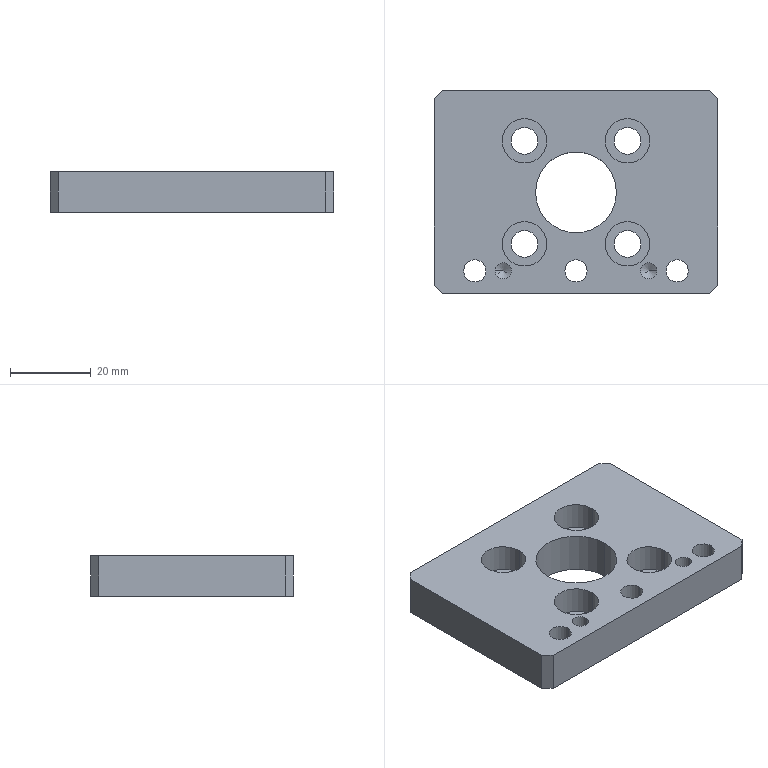Part | SolidWorks | features HoleWzd 3, Chamfer 1, Extrusion 1, ICE 1 | 1 solid | 46 faces | box 70 x 50 x 10 mm | volume 27882 mm3 | cylinder 28 | plane 14 | cone 4 | commonest cylinder face diameters 6.6 x8 11 x8 5.5 x6 4 x4 20 x2
STEP:
#1=CARTESIAN_POINT('',(-20.,-19.5,4.));
#2=VERTEX_POINT('',#1);
#3=CARTESIAN_POINT('',(-16.,-19.5,4.));
#4=VERTEX_POINT('',#3);
#5=CARTESIAN_POINT('',(-18.,-19.5,4.));
#6=DIRECTION('',(0.,0.,1.));
#7=DIRECTION('',(1.,0.,0.));
#8=AXIS2_PLACEMENT_3D('',#5,#6,#7);
#9=CIRCLE('',#8,2.);
#10=EDGE_CURVE('',#2,#4,#9,.T.);
#11=ORIENTED_EDGE('',*,*,#10,.F.);
#12=CARTESIAN_POINT('',(-20.,-19.5,10.));
#13=VERTEX_POINT('',#12);
#14=CARTESIAN_POINT('',(-20.,-19.5,10.));
#15=DIRECTION('',(0.,0.,1.));
#16=VECTOR('',#15,1000.);
#17=LINE('',#14,#16);
#18=EDGE_CURVE('',#2,#13,#17,.T.);
#19=ORIENTED_EDGE('',*,*,#18,.T.);
#20=CARTESIAN_POINT('',(-16.,-19.5,10.));
#21=VERTEX_POINT('',#20);
#22=CARTESIAN_POINT('',(-18.,-19.5,10.));
#23=DIRECTION('',(0.,0.,1.));
#24=DIRECTION('',(1.,0.,0.));
#25=AXIS2_PLACEMENT_3D('',#22,#23,#24);
#26=CIRCLE('',#25,2.);
#27=EDGE_CURVE('',#13,#21,#26,.T.);
#28=ORIENTED_EDGE('',*,*,#27,.T.);
#29=CARTESIAN_POINT('',(-16.,-19.5,10.));
#30=DIRECTION('',(0.,0.,1.));
#31=VECTOR('',#30,1000.);
#32=LINE('',#29,#31);
#33=EDGE_CURVE('',#4,#21,#32,.T.);
#34=ORIENTED_EDGE('',*,*,#33,.F.);
#35=EDGE_LOOP('',(#11,#19,#28,#34));
#36=FACE_OUTER_BOUND('',#35,.T.);
#37=CARTESIAN_POINT('',(-18.,-19.5,10.));
#38=DIRECTION('',(0.,0.,1.));
#39=DIRECTION('',(1.,0.,0.));
#40=AXIS2_PLACEMENT_3D('',#37,#38,#39);
#41=CYLINDRICAL_SURFACE('',#40,2.);
#42=ADVANCED_FACE('',(#36),#41,.F.);
#43=CARTESIAN_POINT('',(-18.,-19.5,2.798));
#44=VERTEX_POINT('',#43);
#45=CARTESIAN_POINT('',(-16.,-19.5,4.));
#46=DIRECTION('',(0.8572,0.,0.515));
#47=VECTOR('',#46,1000.);
#48=LINE('',#45,#47);
#49=EDGE_CURVE('',#44,#4,#48,.T.);
#50=ORIENTED_EDGE('',*,*,#49,.F.);
#51=CARTESIAN_POINT('',(-20.,-19.5,4.));
#52=DIRECTION('',(-0.8572,0.,0.515));
#53=VECTOR('',#52,1000.);
#54=LINE('',#51,#53);
#55=EDGE_CURVE('',#44,#2,#54,.T.);
#56=ORIENTED_EDGE('',*,*,#55,.T.);
#57=ORIENTED_EDGE('',*,*,#10,.T.);
#58=EDGE_LOOP('',(#50,#56,#57));
#59=FACE_OUTER_BOUND('',#58,.T.);
#60=CARTESIAN_POINT('',(-18.,-19.5,4.));
#61=DIRECTION('',(0.,0.,1.));
#62=DIRECTION('',(1.,0.,0.));
#63=AXIS2_PLACEMENT_3D('',#60,#61,#62);
#64=CONICAL_SURFACE('',#63,2.,1.03);
#65=ADVANCED_FACE('',(#59),#64,.F.);
#66=CARTESIAN_POINT('',(16.,-19.5,4.));
#67=VERTEX_POINT('',#66);
#68=CARTESIAN_POINT('',(20.,-19.5,4.));
#69=VERTEX_POINT('',#68);
#70=CARTESIAN_POINT('',(18.,-19.5,4.));
#71=DIRECTION('',(0.,0.,1.));
#72=DIRECTION('',(1.,0.,0.));
#73=AXIS2_PLACEMENT_3D('',#70,#71,#72);
#74=CIRCLE('',#73,2.);
#75=EDGE_CURVE('',#67,#69,#74,.T.);
#76=ORIENTED_EDGE('',*,*,#75,.F.);
#77=CARTESIAN_POINT('',(16.,-19.5,10.));
#78=VERTEX_POINT('',#77);
#79=CARTESIAN_POINT('',(16.,-19.5,10.));
#80=DIRECTION('',(0.,0.,1.));
#81=VECTOR('',#80,1000.);
#82=LINE('',#79,#81);
#83=EDGE_CURVE('',#67,#78,#82,.T.);
#84=ORIENTED_EDGE('',*,*,#83,.T.);
#85=CARTESIAN_POINT('',(20.,-19.5,10.));
#86=VERTEX_POINT('',#85);
#87=CARTESIAN_POINT('',(18.,-19.5,10.));
#88=DIRECTION('',(0.,0.,1.));
#89=DIRECTION('',(1.,0.,0.));
#90=AXIS2_PLACEMENT_3D('',#87,#88,#89);
#91=CIRCLE('',#90,2.);
#92=EDGE_CURVE('',#78,#86,#91,.T.);
#93=ORIENTED_EDGE('',*,*,#92,.T.);
#94=CARTESIAN_POINT('',(20.,-19.5,10.));
#95=DIRECTION('',(0.,0.,1.));
#96=VECTOR('',#95,1000.);
#97=LINE('',#94,#96);
#98=EDGE_CURVE('',#69,#86,#97,.T.);
#99=ORIENTED_EDGE('',*,*,#98,.F.);
#100=EDGE_LOOP('',(#76,#84,#93,#99));
#101=FACE_OUTER_BOUND('',#100,.T.);
#102=CARTESIAN_POINT('',(18.,-19.5,10.));
#103=DIRECTION('',(0.,0.,1.));
#104=DIRECTION('',(1.,0.,0.));
#105=AXIS2_PLACEMENT_3D('',#102,#103,#104);
#106=CYLINDRICAL_SURFACE('',#105,2.);
#107=ADVANCED_FACE('',(#101),#106,.F.);
#108=CARTESIAN_POINT('',(18.,-19.5,2.798));
#109=VERTEX_POINT('',#108);
#110=CARTESIAN_POINT('',(20.,-19.5,4.));
#111=DIRECTION('',(0.8572,0.,0.515));
#112=VECTOR('',#111,1000.);
#113=LINE('',#110,#112);
#114=EDGE_CURVE('',#109,#69,#113,.T.);
#115=ORIENTED_EDGE('',*,*,#114,.F.);
#116=CARTESIAN_POINT('',(16.,-19.5,4.));
#117=DIRECTION('',(-0.8572,0.,0.515));
#118=VECTOR('',#117,1000.);
#119=LINE('',#116,#118);
#120=EDGE_CURVE('',#109,#67,#119,.T.);
#121=ORIENTED_EDGE('',*,*,#120,.T.);
#122=ORIENTED_EDGE('',*,*,#75,.T.);
#123=EDGE_LOOP('',(#115,#121,#122));
#124=FACE_OUTER_BOUND('',#123,.T.);
#125=CARTESIAN_POINT('',(18.,-19.5,4.));
#126=DIRECTION('',(0.,0.,1.));
#127=DIRECTION('',(1.,0.,0.));
#128=AXIS2_PLACEMENT_3D('',#125,#126,#127);
#129=CONICAL_SURFACE('',#128,2.,1.03);
#130=ADVANCED_FACE('',(#124),#129,.F.);
#131=CARTESIAN_POINT('',(-27.75,-19.5,0.));
#132=VERTEX_POINT('',#131);
#133=CARTESIAN_POINT('',(-22.25,-19.5,0.));
#134=VERTEX_POINT('',#133);
#135=CARTESIAN_POINT('',(-25.,-19.5,0.));
#136=DIRECTION('',(0.,0.,1.));
#137=DIRECTION('',(1.,0.,0.));
#138=AXIS2_PLACEMENT_3D('',#135,#136,#137);
#139=CIRCLE('',#138,2.75);
#140=EDGE_CURVE('',#132,#134,#139,.T.);
#141=ORIENTED_EDGE('',*,*,#140,.F.);
#142=CARTESIAN_POINT('',(-27.75,-19.5,10.));
#143=VERTEX_POINT('',#142);
#144=CARTESIAN_POINT('',(-27.75,-19.5,10.));
#145=DIRECTION('',(0.,0.,1.));
#146=VECTOR('',#145,1000.);
#147=LINE('',#144,#146);
#148=EDGE_CURVE('',#132,#143,#147,.T.);
#149=ORIENTED_EDGE('',*,*,#148,.T.);
#150=CARTESIAN_POINT('',(-22.25,-19.5,10.));
#151=VERTEX_POINT('',#150);
#152=CARTESIAN_POINT('',(-25.,-19.5,10.));
#153=DIRECTION('',(0.,0.,1.));
#154=DIRECTION('',(1.,0.,0.));
#155=AXIS2_PLACEMENT_3D('',#152,#153,#154);
#156=CIRCLE('',#155,2.75);
#157=EDGE_CURVE('',#143,#151,#156,.T.);
#158=ORIENTED_EDGE('',*,*,#157,.T.);
#159=CARTESIAN_POINT('',(-22.25,-19.5,10.));
#160=DIRECTION('',(0.,0.,1.));
#161=VECTOR('',#160,1000.);
#162=LINE('',#159,#161);
#163=EDGE_CURVE('',#134,#151,#162,.T.);
#164=ORIENTED_EDGE('',*,*,#163,.F.);
#165=EDGE_LOOP('',(#141,#149,#158,#164));
#166=FACE_OUTER_BOUND('',#165,.T.);
#167=CARTESIAN_POINT('',(-25.,-19.5,10.));
#168=DIRECTION('',(0.,0.,1.));
#169=DIRECTION('',(1.,0.,0.));
#170=AXIS2_PLACEMENT_3D('',#167,#168,#169);
#171=CYLINDRICAL_SURFACE('',#170,2.75);
#172=ADVANCED_FACE('',(#166),#171,.F.);
#173=CARTESIAN_POINT('',(-2.75,-19.5,0.));
#174=VERTEX_POINT('',#173);
#175=CARTESIAN_POINT('',(2.75,-19.5,0.));
#176=VERTEX_POINT('',#175);
#177=CARTESIAN_POINT('',(0.,-19.5,0.));
#178=DIRECTION('',(0.,0.,1.));
#179=DIRECTION('',(1.,0.,0.));
#180=AXIS2_PLACEMENT_3D('',#177,#178,#179);
#181=CIRCLE('',#180,2.75);
#182=EDGE_CURVE('',#174,#176,#181,.T.);
#183=ORIENTED_EDGE('',*,*,#182,.F.);
#184=CARTESIAN_POINT('',(-2.75,-19.5,10.));
#185=VERTEX_POINT('',#184);
#186=CARTESIAN_POINT('',(-2.75,-19.5,10.));
#187=DIRECTION('',(0.,0.,1.));
#188=VECTOR('',#187,1000.);
#189=LINE('',#186,#188);
#190=EDGE_CURVE('',#174,#185,#189,.T.);
#191=ORIENTED_EDGE('',*,*,#190,.T.);
#192=CARTESIAN_POINT('',(2.75,-19.5,10.));
#193=VERTEX_POINT('',#192);
#194=CARTESIAN_POINT('',(0.,-19.5,10.));
#195=DIRECTION('',(0.,0.,1.));
#196=DIRECTION('',(1.,0.,0.));
#197=AXIS2_PLACEMENT_3D('',#194,#195,#196);
#198=CIRCLE('',#197,2.75);
#199=EDGE_CURVE('',#185,#193,#198,.T.);
#200=ORIENTED_EDGE('',*,*,#199,.T.);
#201=CARTESIAN_POINT('',(2.75,-19.5,10.));
#202=DIRECTION('',(0.,0.,1.));
#203=VECTOR('',#202,1000.);
#204=LINE('',#201,#203);
#205=EDGE_CURVE('',#176,#193,#204,.T.);
#206=ORIENTED_EDGE('',*,*,#205,.F.);
#207=EDGE_LOOP('',(#183,#191,#200,#206));
#208=FACE_OUTER_BOUND('',#207,.T.);
#209=CARTESIAN_POINT('',(0.,-19.5,10.));
#210=DIRECTION('',(0.,0.,1.));
#211=DIRECTION('',(1.,0.,0.));
#212=AXIS2_PLACEMENT_3D('',#209,#210,#211);
#213=CYLINDRICAL_SURFACE('',#212,2.75);
#214=ADVANCED_FACE('',(#208),#213,.F.);
#215=CARTESIAN_POINT('',(22.25,-19.5,0.));
#216=VERTEX_POINT('',#215);
#217=CARTESIAN_POINT('',(27.75,-19.5,0.));
#218=VERTEX_POINT('',#217);
#219=CARTESIAN_POINT('',(25.,-19.5,0.));
#220=DIRECTION('',(0.,0.,1.));
#221=DIRECTION('',(1.,0.,0.));
#222=AXIS2_PLACEMENT_3D('',#219,#220,#221);
#223=CIRCLE('',#222,2.75);
#224=EDGE_CURVE('',#216,#218,#223,.T.);
#225=ORIENTED_EDGE('',*,*,#224,.F.);
#226=CARTESIAN_POINT('',(22.25,-19.5,10.));
#227=VERTEX_POINT('',#226);
#228=CARTESIAN_POINT('',(22.25,-19.5,10.));
#229=DIRECTION('',(0.,0.,1.));
#230=VECTOR('',#229,1000.);
#231=LINE('',#228,#230);
#232=EDGE_CURVE('',#216,#227,#231,.T.);
#233=ORIENTED_EDGE('',*,*,#232,.T.);
#234=CARTESIAN_POINT('',(27.75,-19.5,10.));
#235=VERTEX_POINT('',#234);
#236=CARTESIAN_POINT('',(25.,-19.5,10.));
#237=DIRECTION('',(0.,0.,1.));
#238=DIRECTION('',(1.,0.,0.));
#239=AXIS2_PLACEMENT_3D('',#236,#237,#238);
#240=CIRCLE('',#239,2.75);
#241=EDGE_CURVE('',#227,#235,#240,.T.);
#242=ORIENTED_EDGE('',*,*,#241,.T.);
#243=CARTESIAN_POINT('',(27.75,-19.5,10.));
#244=DIRECTION('',(0.,0.,1.));
#245=VECTOR('',#244,1000.);
#246=LINE('',#243,#245);
#247=EDGE_CURVE('',#218,#235,#246,.T.);
#248=ORIENTED_EDGE('',*,*,#247,.F.);
#249=EDGE_LOOP('',(#225,#233,#242,#248));
#250=FACE_OUTER_BOUND('',#249,.T.);
#251=CARTESIAN_POINT('',(25.,-19.5,10.));
#252=DIRECTION('',(0.,0.,1.));
#253=DIRECTION('',(1.,0.,0.));
#254=AXIS2_PLACEMENT_3D('',#251,#252,#253);
#255=CYLINDRICAL_SURFACE('',#254,2.75);
#256=ADVANCED_FACE('',(#250),#255,.F.);
#257=CARTESIAN_POINT('',(-18.228,12.628,3.2));
#258=VERTEX_POINT('',#257);
#259=CARTESIAN_POINT('',(-7.228,12.628,3.2));
#260=VERTEX_POINT('',#259);
#261=CARTESIAN_POINT('',(-12.728,12.628,3.2));
#262=DIRECTION('',(0.,0.,1.));
#263=DIRECTION('',(1.,0.,0.));
#264=AXIS2_PLACEMENT_3D('',#261,#262,#263);
#265=CIRCLE('',#264,5.5);
#266=EDGE_CURVE('',#258,#260,#265,.T.);
#267=ORIENTED_EDGE('',*,*,#266,.F.);
#268=CARTESIAN_POINT('',(-18.228,12.628,10.));
#269=VERTEX_POINT('',#268);
#270=CARTESIAN_POINT('',(-18.228,12.628,10.));
#271=DIRECTION('',(0.,0.,1.));
#272=VECTOR('',#271,1000.);
#273=LINE('',#270,#272);
#274=EDGE_CURVE('',#258,#269,#273,.T.);
#275=ORIENTED_EDGE('',*,*,#274,.T.);
#276=CARTESIAN_POINT('',(-7.228,12.628,10.));
#277=VERTEX_POINT('',#276);
#278=CARTESIAN_POINT('',(-12.728,12.628,10.));
#279=DIRECTION('',(0.,0.,1.));
#280=DIRECTION('',(1.,0.,0.));
#281=AXIS2_PLACEMENT_3D('',#278,#279,#280);
#282=CIRCLE('',#281,5.5);
#283=EDGE_CURVE('',#269,#277,#282,.T.);
#284=ORIENTED_EDGE('',*,*,#283,.T.);
#285=CARTESIAN_POINT('',(-7.228,12.628,10.));
#286=DIRECTION('',(0.,0.,1.));
#287=VECTOR('',#286,1000.);
#288=LINE('',#285,#287);
#289=EDGE_CURVE('',#260,#277,#288,.T.);
#290=ORIENTED_EDGE('',*,*,#289,.F.);
#291=EDGE_LOOP('',(#267,#275,#284,#290));
#292=FACE_OUTER_BOUND('',#291,.T.);
#293=CARTESIAN_POINT('',(-12.728,12.628,10.));
#294=DIRECTION('',(0.,0.,1.));
#295=DIRECTION('',(1.,0.,0.));
#296=AXIS2_PLACEMENT_3D('',#293,#294,#295);
#297=CYLINDRICAL_SURFACE('',#296,5.5);
#298=ADVANCED_FACE('',(#292),#297,.F.);
#299=CARTESIAN_POINT('',(-16.028,12.628,0.));
#300=VERTEX_POINT('',#299);
#301=CARTESIAN_POINT('',(-9.428,12.628,0.));
#302=VERTEX_POINT('',#301);
#303=CARTESIAN_POINT('',(-12.728,12.628,0.));
#304=DIRECTION('',(0.,0.,1.));
#305=DIRECTION('',(1.,0.,0.));
#306=AXIS2_PLACEMENT_3D('',#303,#304,#305);
#307=CIRCLE('',#306,3.3);
#308=EDGE_CURVE('',#300,#302,#307,.T.);
#309=ORIENTED_EDGE('',*,*,#308,.F.);
#310=CARTESIAN_POINT('',(-16.028,12.628,3.2));
#311=VERTEX_POINT('',#310);
#312=CARTESIAN_POINT('',(-16.028,12.628,10.));
#313=DIRECTION('',(0.,0.,1.));
#314=VECTOR('',#313,1000.);
#315=LINE('',#312,#314);
#316=EDGE_CURVE('',#300,#311,#315,.T.);
#317=ORIENTED_EDGE('',*,*,#316,.T.);
#318=CARTESIAN_POINT('',(-9.428,12.628,3.2));
#319=VERTEX_POINT('',#318);
#320=CARTESIAN_POINT('',(-12.728,12.628,3.2));
#321=DIRECTION('',(0.,0.,1.));
#322=DIRECTION('',(1.,0.,0.));
#323=AXIS2_PLACEMENT_3D('',#320,#321,#322);
#324=CIRCLE('',#323,3.3);
#325=EDGE_CURVE('',#311,#319,#324,.T.);
#326=ORIENTED_EDGE('',*,*,#325,.T.);
#327=CARTESIAN_POINT('',(-9.428,12.628,10.));
#328=DIRECTION('',(0.,0.,1.));
#329=VECTOR('',#328,1000.);
#330=LINE('',#327,#329);
#331=EDGE_CURVE('',#302,#319,#330,.T.);
#332=ORIENTED_EDGE('',*,*,#331,.F.);
#333=EDGE_LOOP('',(#309,#317,#326,#332));
#334=FACE_OUTER_BOUND('',#333,.T.);
#335=CARTESIAN_POINT('',(-12.728,12.628,10.));
#336=DIRECTION('',(0.,0.,1.));
#337=DIRECTION('',(1.,0.,0.));
#338=AXIS2_PLACEMENT_3D('',#335,#336,#337);
#339=CYLINDRICAL_SURFACE('',#338,3.3);
#340=ADVANCED_FACE('',(#334),#339,.F.);
#341=CARTESIAN_POINT('',(7.228,-12.828,3.2));
#342=VERTEX_POINT('',#341);
#343=CARTESIAN_POINT('',(18.228,-12.828,3.2));
#344=VERTEX_POINT('',#343);
#345=CARTESIAN_POINT('',(12.728,-12.828,3.2));
#346=DIRECTION('',(0.,0.,1.));
#347=DIRECTION('',(1.,0.,0.));
#348=AXIS2_PLACEMENT_3D('',#345,#346,#347);
#349=CIRCLE('',#348,5.5);
#350=EDGE_CURVE('',#342,#344,#349,.T.);
#351=ORIENTED_EDGE('',*,*,#350,.F.);
#352=CARTESIAN_POINT('',(7.228,-12.828,10.));
#353=VERTEX_POINT('',#352);
#354=CARTESIAN_POINT('',(7.228,-12.828,10.));
#355=DIRECTION('',(0.,0.,1.));
#356=VECTOR('',#355,1000.);
#357=LINE('',#354,#356);
#358=EDGE_CURVE('',#342,#353,#357,.T.);
#359=ORIENTED_EDGE('',*,*,#358,.T.);
#360=CARTESIAN_POINT('',(18.228,-12.828,10.));
#361=VERTEX_POINT('',#360);
#362=CARTESIAN_POINT('',(12.728,-12.828,10.));
#363=DIRECTION('',(0.,0.,1.));
#364=DIRECTION('',(1.,0.,0.));
#365=AXIS2_PLACEMENT_3D('',#362,#363,#364);
#366=CIRCLE('',#365,5.5);
#367=EDGE_CURVE('',#353,#361,#366,.T.);
#368=ORIENTED_EDGE('',*,*,#367,.T.);
#369=CARTESIAN_POINT('',(18.228,-12.828,10.));
#370=DIRECTION('',(0.,0.,1.));
#371=VECTOR('',#370,1000.);
#372=LINE('',#369,#371);
#373=EDGE_CURVE('',#344,#361,#372,.T.);
#374=ORIENTED_EDGE('',*,*,#373,.F.);
#375=EDGE_LOOP('',(#351,#359,#368,#374));
#376=FACE_OUTER_BOUND('',#375,.T.);
#377=CARTESIAN_POINT('',(12.728,-12.828,10.));
#378=DIRECTION('',(0.,0.,1.));
#379=DIRECTION('',(1.,0.,0.));
#380=AXIS2_PLACEMENT_3D('',#377,#378,#379);
#381=CYLINDRICAL_SURFACE('',#380,5.5);
#382=ADVANCED_FACE('',(#376),#381,.F.);
#383=CARTESIAN_POINT('',(9.428,-12.828,0.));
#384=VERTEX_POINT('',#383);
#385=CARTESIAN_POINT('',(16.028,-12.828,0.));
#386=VERTEX_POINT('',#385);
#387=CARTESIAN_POINT('',(12.728,-12.828,0.));
#388=DIRECTION('',(0.,0.,1.));
#389=DIRECTION('',(1.,0.,0.));
#390=AXIS2_PLACEMENT_3D('',#387,#388,#389);
#391=CIRCLE('',#390,3.3);
#392=EDGE_CURVE('',#384,#386,#391,.T.);
#393=ORIENTED_EDGE('',*,*,#392,.F.);
#394=CARTESIAN_POINT('',(9.428,-12.828,3.2));
#395=VERTEX_POINT('',#394);
#396=CARTESIAN_POINT('',(9.428,-12.828,10.));
#397=DIRECTION('',(0.,0.,1.));
#398=VECTOR('',#397,1000.);
#399=LINE('',#396,#398);
#400=EDGE_CURVE('',#384,#395,#399,.T.);
#401=ORIENTED_EDGE('',*,*,#400,.T.);
#402=CARTESIAN_POINT('',(16.028,-12.828,3.2));
#403=VERTEX_POINT('',#402);
#404=CARTESIAN_POINT('',(12.728,-12.828,3.2));
#405=DIRECTION('',(0.,0.,1.));
#406=DIRECTION('',(1.,0.,0.));
#407=AXIS2_PLACEMENT_3D('',#404,#405,#406);
#408=CIRCLE('',#407,3.3);
#409=EDGE_CURVE('',#395,#403,#408,.T.);
#410=ORIENTED_EDGE('',*,*,#409,.T.);
#411=CARTESIAN_POINT('',(16.028,-12.828,10.));
#412=DIRECTION('',(0.,0.,1.));
#413=VECTOR('',#412,1000.);
#414=LINE('',#411,#413);
#415=EDGE_CURVE('',#386,#403,#414,.T.);
#416=ORIENTED_EDGE('',*,*,#415,.F.);
#417=EDGE_LOOP('',(#393,#401,#410,#416));
#418=FACE_OUTER_BOUND('',#417,.T.);
#419=CARTESIAN_POINT('',(12.728,-12.828,10.));
#420=DIRECTION('',(0.,0.,1.));
#421=DIRECTION('',(1.,0.,0.));
#422=AXIS2_PLACEMENT_3D('',#419,#420,#421);
#423=CYLINDRICAL_SURFACE('',#422,3.3);
#424=ADVANCED_FACE('',(#418),#423,.F.);
#425=CARTESIAN_POINT('',(-18.228,-12.828,3.2));
#426=VERTEX_POINT('',#425);
#427=CARTESIAN_POINT('',(-7.228,-12.828,3.2));
#428=VERTEX_POINT('',#427);
#429=CARTESIAN_POINT('',(-12.728,-12.828,3.2));
#430=DIRECTION('',(0.,0.,1.));
#431=DIRECTION('',(1.,0.,0.));
#432=AXIS2_PLACEMENT_3D('',#429,#430,#431);
#433=CIRCLE('',#432,5.5);
#434=EDGE_CURVE('',#426,#428,#433,.T.);
#435=ORIENTED_EDGE('',*,*,#434,.F.);
#436=CARTESIAN_POINT('',(-18.228,-12.828,10.));
#437=VERTEX_POINT('',#436);
#438=CARTESIAN_POINT('',(-18.228,-12.828,10.));
#439=DIRECTION('',(0.,0.,1.));
#440=VECTOR('',#439,1000.);
#441=LINE('',#438,#440);
#442=EDGE_CURVE('',#426,#437,#441,.T.);
#443=ORIENTED_EDGE('',*,*,#442,.T.);
#444=CARTESIAN_POINT('',(-7.228,-12.828,10.));
#445=VERTEX_POINT('',#444);
#446=CARTESIAN_POINT('',(-12.728,-12.828,10.));
#447=DIRECTION('',(0.,0.,1.));
#448=DIRECTION('',(1.,0.,0.));
#449=AXIS2_PLACEMENT_3D('',#446,#447,#448);
#450=CIRCLE('',#449,5.5);
#451=EDGE_CURVE('',#437,#445,#450,.T.);
#452=ORIENTED_EDGE('',*,*,#451,.T.);
#453=CARTESIAN_POINT('',(-7.228,-12.828,10.));
#454=DIRECTION('',(0.,0.,1.));
#455=VECTOR('',#454,1000.);
#456=LINE('',#453,#455);
#457=EDGE_CURVE('',#428,#445,#456,.T.);
#458=ORIENTED_EDGE('',*,*,#457,.F.);
#459=EDGE_LOOP('',(#435,#443,#452,#458));
#460=FACE_OUTER_BOUND('',#459,.T.);
#461=CARTESIAN_POINT('',(-12.728,-12.828,10.));
#462=DIRECTION('',(0.,0.,1.));
#463=DIRECTION('',(1.,0.,0.));
#464=AXIS2_PLACEMENT_3D('',#461,#462,#463);
#465=CYLINDRICAL_SURFACE('',#464,5.5);
#466=ADVANCED_FACE('',(#460),#465,.F.);
#467=CARTESIAN_POINT('',(-16.028,-12.828,0.));
#468=VERTEX_POINT('',#467);
#469=CARTESIAN_POINT('',(-9.428,-12.828,0.));
#470=VERTEX_POINT('',#469);
#471=CARTESIAN_POINT('',(-12.728,-12.828,0.));
#472=DIRECTION('',(0.,0.,1.));
#473=DIRECTION('',(1.,0.,0.));
#474=AXIS2_PLACEMENT_3D('',#471,#472,#473);
#475=CIRCLE('',#474,3.3);
#476=EDGE_CURVE('',#468,#470,#475,.T.);
#477=ORIENTED_EDGE('',*,*,#476,.F.);
#478=CARTESIAN_POINT('',(-16.028,-12.828,3.2));
#479=VERTEX_POINT('',#478);
#480=CARTESIAN_POINT('',(-16.028,-12.828,10.));
#481=DIRECTION('',(0.,0.,1.));
#482=VECTOR('',#481,1000.);
#483=LINE('',#480,#482);
#484=EDGE_CURVE('',#468,#479,#483,.T.);
#485=ORIENTED_EDGE('',*,*,#484,.T.);
#486=CARTESIAN_POINT('',(-9.428,-12.828,3.2));
#487=VERTEX_POINT('',#486);
#488=CARTESIAN_POINT('',(-12.728,-12.828,3.2));
#489=DIRECTION('',(0.,0.,1.));
#490=DIRECTION('',(1.,0.,0.));
#491=AXIS2_PLACEMENT_3D('',#488,#489,#490);
#492=CIRCLE('',#491,3.3);
#493=EDGE_CURVE('',#479,#487,#492,.T.);
#494=ORIENTED_EDGE('',*,*,#493,.T.);
#495=CARTESIAN_POINT('',(-9.428,-12.828,10.));
#496=DIRECTION('',(0.,0.,1.));
#497=VECTOR('',#496,1000.);
#498=LINE('',#495,#497);
#499=EDGE_CURVE('',#470,#487,#498,.T.);
#500=ORIENTED_EDGE('',*,*,#499,.F.);
#501=EDGE_LOOP('',(#477,#485,#494,#500));
#502=FACE_OUTER_BOUND('',#501,.T.);
#503=CARTESIAN_POINT('',(-12.728,-12.828,10.));
#504=DIRECTION('',(0.,0.,1.));
#505=DIRECTION('',(1.,0.,0.));
#506=AXIS2_PLACEMENT_3D('',#503,#504,#505);
#507=CYLINDRICAL_SURFACE('',#506,3.3);
#508=ADVANCED_FACE('',(#502),#507,.F.);
#509=CARTESIAN_POINT('',(7.228,12.628,3.2));
#510=VERTEX_POINT('',#509);
#511=CARTESIAN_POINT('',(18.228,12.628,3.2));
#512=VERTEX_POINT('',#511);
#513=CARTESIAN_POINT('',(12.728,12.628,3.2));
#514=DIRECTION('',(0.,0.,1.));
#515=DIRECTION('',(1.,0.,0.));
#516=AXIS2_PLACEMENT_3D('',#513,#514,#515);
#517=CIRCLE('',#516,5.5);
#518=EDGE_CURVE('',#510,#512,#517,.T.);
#519=ORIENTED_EDGE('',*,*,#518,.F.);
#520=CARTESIAN_POINT('',(7.228,12.628,10.));
#521=VERTEX_POINT('',#520);
#522=CARTESIAN_POINT('',(7.228,12.628,10.));
#523=DIRECTION('',(0.,0.,1.));
#524=VECTOR('',#523,1000.);
#525=LINE('',#522,#524);
#526=EDGE_CURVE('',#510,#521,#525,.T.);
#527=ORIENTED_EDGE('',*,*,#526,.T.);
#528=CARTESIAN_POINT('',(18.228,12.628,10.));
#529=VERTEX_POINT('',#528);
#530=CARTESIAN_POINT('',(12.728,12.628,10.));
#531=DIRECTION('',(0.,0.,1.));
#532=DIRECTION('',(1.,0.,0.));
#533=AXIS2_PLACEMENT_3D('',#530,#531,#532);
#534=CIRCLE('',#533,5.5);
#535=EDGE_CURVE('',#521,#529,#534,.T.);
#536=ORIENTED_EDGE('',*,*,#535,.T.);
#537=CARTESIAN_POINT('',(18.228,12.628,10.));
#538=DIRECTION('',(0.,0.,1.));
#539=VECTOR('',#538,1000.);
#540=LINE('',#537,#539);
#541=EDGE_CURVE('',#512,#529,#540,.T.);
#542=ORIENTED_EDGE('',*,*,#541,.F.);
#543=EDGE_LOOP('',(#519,#527,#536,#542));
#544=FACE_OUTER_BOUND('',#543,.T.);
#545=CARTESIAN_POINT('',(12.728,12.628,10.));
#546=DIRECTION('',(0.,0.,1.));
#547=DIRECTION('',(1.,0.,0.));
#548=AXIS2_PLACEMENT_3D('',#545,#546,#547);
#549=CYLINDRICAL_SURFACE('',#548,5.5);
#550=ADVANCED_FACE('',(#544),#549,.F.);
#551=CARTESIAN_POINT('',(9.428,12.628,0.));
#552=VERTEX_POINT('',#551);
#553=CARTESIAN_POINT('',(16.028,12.628,0.));
#554=VERTEX_POINT('',#553);
#555=CARTESIAN_POINT('',(12.728,12.628,0.));
#556=DIRECTION('',(0.,0.,1.));
#557=DIRECTION('',(1.,0.,0.));
#558=AXIS2_PLACEMENT_3D('',#555,#556,#557);
#559=CIRCLE('',#558,3.3);
#560=EDGE_CURVE('',#552,#554,#559,.T.);
#561=ORIENTED_EDGE('',*,*,#560,.F.);
#562=CARTESIAN_POINT('',(9.428,12.628,3.2));
#563=VERTEX_POINT('',#562);
#564=CARTESIAN_POINT('',(9.428,12.628,10.));
#565=DIRECTION('',(0.,0.,1.));
#566=VECTOR('',#565,1000.);
#567=LINE('',#564,#566);
#568=EDGE_CURVE('',#552,#563,#567,.T.);
#569=ORIENTED_EDGE('',*,*,#568,.T.);
#570=CARTESIAN_POINT('',(16.028,12.628,3.2));
#571=VERTEX_POINT('',#570);
#572=CARTESIAN_POINT('',(12.728,12.628,3.2));
#573=DIRECTION('',(0.,0.,1.));
#574=DIRECTION('',(1.,0.,0.));
#575=AXIS2_PLACEMENT_3D('',#572,#573,#574);
#576=CIRCLE('',#575,3.3);
#577=EDGE_CURVE('',#563,#571,#576,.T.);
#578=ORIENTED_EDGE('',*,*,#577,.T.);
#579=CARTESIAN_POINT('',(16.028,12.628,10.));
#580=DIRECTION('',(0.,0.,1.));
#581=VECTOR('',#580,1000.);
#582=LINE('',#579,#581);
#583=EDGE_CURVE('',#554,#571,#582,.T.);
#584=ORIENTED_EDGE('',*,*,#583,.F.);
#585=EDGE_LOOP('',(#561,#569,#578,#584));
#586=FACE_OUTER_BOUND('',#585,.T.);
#587=CARTESIAN_POINT('',(12.728,12.628,10.));
#588=DIRECTION('',(0.,0.,1.));
#589=DIRECTION('',(1.,0.,0.));
#590=AXIS2_PLACEMENT_3D('',#587,#588,#589);
#591=CYLINDRICAL_SURFACE('',#590,3.3);
#592=ADVANCED_FACE('',(#586),#591,.F.);
#593=CARTESIAN_POINT('',(-10.,-0.1,0.));
#594=VERTEX_POINT('',#593);
#595=CARTESIAN_POINT('',(10.,-0.1,0.));
#596=VERTEX_POINT('',#595);
#597=CARTESIAN_POINT('',(0.,-0.1,0.));
#598=DIRECTION('',(0.,0.,1.));
#599=DIRECTION('',(1.,0.,0.));
#600=AXIS2_PLACEMENT_3D('',#597,#598,#599);
#601=CIRCLE('',#600,10.);
#602=EDGE_CURVE('',#594,#596,#601,.T.);
#603=ORIENTED_EDGE('',*,*,#602,.F.);
#604=CARTESIAN_POINT('',(-10.,-0.1,10.));
#605=VERTEX_POINT('',#604);
#606=CARTESIAN_POINT('',(-10.,-0.1,0.));
#607=DIRECTION('',(0.,0.,1.));
#608=VECTOR('',#607,1000.);
#609=LINE('',#606,#608);
#610=EDGE_CURVE('',#594,#605,#609,.T.);
#611=ORIENTED_EDGE('',*,*,#610,.T.);
#612=CARTESIAN_POINT('',(10.,-0.1,10.));
#613=VERTEX_POINT('',#612);
#614=CARTESIAN_POINT('',(0.,-0.1,10.));
#615=DIRECTION('',(0.,0.,1.));
#616=DIRECTION('',(1.,0.,0.));
#617=AXIS2_PLACEMENT_3D('',#614,#615,#616);
#618=CIRCLE('',#617,10.);
#619=EDGE_CURVE('',#605,#613,#618,.T.);
#620=ORIENTED_EDGE('',*,*,#619,.T.);
#621=CARTESIAN_POINT('',(10.,-0.1,0.));
#622=DIRECTION('',(0.,0.,1.));
#623=VECTOR('',#622,1000.);
#624=LINE('',#621,#623);
#625=EDGE_CURVE('',#596,#613,#624,.T.);
#626=ORIENTED_EDGE('',*,*,#625,.F.);
#627=EDGE_LOOP('',(#603,#611,#620,#626));
#628=FACE_OUTER_BOUND('',#627,.T.);
#629=CARTESIAN_POINT('',(0.,-0.1,0.));
#630=DIRECTION('',(0.,0.,1.));
#631=DIRECTION('',(1.,0.,0.));
#632=AXIS2_PLACEMENT_3D('',#629,#630,#631);
#633=CYLINDRICAL_SURFACE('',#632,10.);
#634=ADVANCED_FACE('',(#628),#633,.F.);
#635=CARTESIAN_POINT('',(35.,-23.,0.));
#636=VERTEX_POINT('',#635);
#637=CARTESIAN_POINT('',(35.,23.,0.));
#638=VERTEX_POINT('',#637);
#639=CARTESIAN_POINT('',(35.,25.,0.));
#640=DIRECTION('',(0.,1.,0.));
#641=VECTOR('',#640,1000.);
#642=LINE('',#639,#641);
#643=EDGE_CURVE('',#636,#638,#642,.T.);
#644=ORIENTED_EDGE('',*,*,#643,.T.);
#645=CARTESIAN_POINT('',(35.,23.,10.));
#646=VERTEX_POINT('',#645);
#647=CARTESIAN_POINT('',(35.,23.,10.));
#648=DIRECTION('',(0.,0.,1.));
#649=VECTOR('',#648,1000.);
#650=LINE('',#647,#649);
#651=EDGE_CURVE('',#638,#646,#650,.T.);
#652=ORIENTED_EDGE('',*,*,#651,.T.);
#653=CARTESIAN_POINT('',(35.,-23.,10.));
#654=VERTEX_POINT('',#653);
#655=CARTESIAN_POINT('',(35.,25.,10.));
#656=DIRECTION('',(0.,1.,0.));
#657=VECTOR('',#656,1000.);
#658=LINE('',#655,#657);
#659=EDGE_CURVE('',#654,#646,#658,.T.);
#660=ORIENTED_EDGE('',*,*,#659,.F.);
#661=CARTESIAN_POINT('',(35.,-23.,10.));
#662=DIRECTION('',(0.,0.,-1.));
#663=VECTOR('',#662,1000.);
#664=LINE('',#661,#663);
#665=EDGE_CURVE('',#654,#636,#664,.T.);
#666=ORIENTED_EDGE('',*,*,#665,.T.);
#667=EDGE_LOOP('',(#644,#652,#660,#666));
#668=FACE_OUTER_BOUND('',#667,.T.);
#669=CARTESIAN_POINT('',(35.,25.,10.));
#670=DIRECTION('',(-1.,0.,0.));
#671=DIRECTION('',(0.,-1.,0.));
#672=AXIS2_PLACEMENT_3D('',#669,#670,#671);
#673=PLANE('',#672);
#674=ADVANCED_FACE('',(#668),#673,.F.);
#675=CARTESIAN_POINT('',(33.,25.,10.));
#676=VERTEX_POINT('',#675);
#677=CARTESIAN_POINT('',(-33.,25.,10.));
#678=VERTEX_POINT('',#677);
#679=CARTESIAN_POINT('',(-35.,25.,10.));
#680=DIRECTION('',(-1.,0.,0.));
#681=VECTOR('',#680,1000.);
#682=LINE('',#679,#681);
#683=EDGE_CURVE('',#676,#678,#682,.T.);
#684=ORIENTED_EDGE('',*,*,#683,.F.);
#685=CARTESIAN_POINT('',(33.,25.,0.));
#686=VERTEX_POINT('',#685);
#687=CARTESIAN_POINT('',(33.,25.,10.));
#688=DIRECTION('',(0.,0.,-1.));
#689=VECTOR('',#688,1000.);
#690=LINE('',#687,#689);
#691=EDGE_CURVE('',#676,#686,#690,.T.);
#692=ORIENTED_EDGE('',*,*,#691,.T.);
#693=CARTESIAN_POINT('',(-33.,25.,0.));
#694=VERTEX_POINT('',#693);
#695=CARTESIAN_POINT('',(-35.,25.,0.));
#696=DIRECTION('',(-1.,0.,0.));
#697=VECTOR('',#696,1000.);
#698=LINE('',#695,#697);
#699=EDGE_CURVE('',#686,#694,#698,.T.);
#700=ORIENTED_EDGE('',*,*,#699,.T.);
#701=CARTESIAN_POINT('',(-33.,25.,10.));
#702=DIRECTION('',(0.,0.,1.));
#703=VECTOR('',#702,1000.);
#704=LINE('',#701,#703);
#705=EDGE_CURVE('',#694,#678,#704,.T.);
#706=ORIENTED_EDGE('',*,*,#705,.T.);
#707=EDGE_LOOP('',(#684,#692,#700,#706));
#708=FACE_OUTER_BOUND('',#707,.T.);
#709=CARTESIAN_POINT('',(-35.,25.,10.));
#710=DIRECTION('',(0.,-1.,0.));
#711=DIRECTION('',(0.,0.,-1.));
#712=AXIS2_PLACEMENT_3D('',#709,#710,#711);
#713=PLANE('',#712);
#714=ADVANCED_FACE('',(#708),#713,.F.);
#715=CARTESIAN_POINT('',(-35.,23.,0.));
#716=VERTEX_POINT('',#715);
#717=CARTESIAN_POINT('',(-35.,-23.,0.));
#718=VERTEX_POINT('',#717);
#719=CARTESIAN_POINT('',(-35.,25.,0.));
#720=DIRECTION('',(0.,-1.,0.));
#721=VECTOR('',#720,1000.);
#722=LINE('',#719,#721);
#723=EDGE_CURVE('',#716,#718,#722,.T.);
#724=ORIENTED_EDGE('',*,*,#723,.T.);
#725=CARTESIAN_POINT('',(-35.,-23.,10.));
#726=VERTEX_POINT('',#725);
#727=CARTESIAN_POINT('',(-35.,-23.,10.));
#728=DIRECTION('',(0.,0.,1.));
#729=VECTOR('',#728,1000.);
#730=LINE('',#727,#729);
#731=EDGE_CURVE('',#718,#726,#730,.T.);
#732=ORIENTED_EDGE('',*,*,#731,.T.);
#733=CARTESIAN_POINT('',(-35.,23.,10.));
#734=VERTEX_POINT('',#733);
#735=CARTESIAN_POINT('',(-35.,25.,10.));
#736=DIRECTION('',(0.,-1.,0.));
#737=VECTOR('',#736,1000.);
#738=LINE('',#735,#737);
#739=EDGE_CURVE('',#734,#726,#738,.T.);
#740=ORIENTED_EDGE('',*,*,#739,.F.);
#741=CARTESIAN_POINT('',(-35.,23.,10.));
#742=DIRECTION('',(0.,0.,-1.));
#743=VECTOR('',#742,1000.);
#744=LINE('',#741,#743);
#745=EDGE_CURVE('',#734,#716,#744,.T.);
#746=ORIENTED_EDGE('',*,*,#745,.T.);
#747=EDGE_LOOP('',(#724,#732,#740,#746));
#748=FACE_OUTER_BOUND('',#747,.T.);
#749=CARTESIAN_POINT('',(-35.,25.,10.));
#750=DIRECTION('',(1.,0.,0.));
#751=DIRECTION('',(0.,1.,0.));
#752=AXIS2_PLACEMENT_3D('',#749,#750,#751);
#753=PLANE('',#752);
#754=ADVANCED_FACE('',(#748),#753,.F.);
#755=CARTESIAN_POINT('',(-33.,-25.,0.));
#756=VERTEX_POINT('',#755);
#757=CARTESIAN_POINT('',(33.,-25.,0.));
#758=VERTEX_POINT('',#757);
#759=CARTESIAN_POINT('',(-35.,-25.,0.));
#760=DIRECTION('',(1.,0.,0.));
#761=VECTOR('',#760,1000.);
#762=LINE('',#759,#761);
#763=EDGE_CURVE('',#756,#758,#762,.T.);
#764=ORIENTED_EDGE('',*,*,#763,.T.);
#765=CARTESIAN_POINT('',(33.,-25.,10.));
#766=VERTEX_POINT('',#765);
#767=CARTESIAN_POINT('',(33.,-25.,10.));
#768=DIRECTION('',(0.,0.,1.));
#769=VECTOR('',#768,1000.);
#770=LINE('',#767,#769);
#771=EDGE_CURVE('',#758,#766,#770,.T.);
#772=ORIENTED_EDGE('',*,*,#771,.T.);
#773=CARTESIAN_POINT('',(-33.,-25.,10.));
#774=VERTEX_POINT('',#773);
#775=CARTESIAN_POINT('',(-35.,-25.,10.));
#776=DIRECTION('',(1.,0.,0.));
#777=VECTOR('',#776,1000.);
#778=LINE('',#775,#777);
#779=EDGE_CURVE('',#774,#766,#778,.T.);
#780=ORIENTED_EDGE('',*,*,#779,.F.);
#781=CARTESIAN_POINT('',(-33.,-25.,10.));
#782=DIRECTION('',(0.,0.,-1.));
#783=VECTOR('',#782,1000.);
#784=LINE('',#781,#783);
#785=EDGE_CURVE('',#774,#756,#784,.T.);
#786=ORIENTED_EDGE('',*,*,#785,.T.);
#787=EDGE_LOOP('',(#764,#772,#780,#786));
#788=FACE_OUTER_BOUND('',#787,.T.);
#789=CARTESIAN_POINT('',(-35.,-25.,10.));
#790=DIRECTION('',(0.,1.,0.));
#791=DIRECTION('',(0.,0.,1.));
#792=AXIS2_PLACEMENT_3D('',#789,#790,#791);
#793=PLANE('',#792);
#794=ADVANCED_FACE('',(#788),#793,.F.);
#795=CARTESIAN_POINT('',(-18.,-19.5,10.));
#796=DIRECTION('',(0.,0.,1.));
#797=DIRECTION('',(1.,0.,0.));
#798=AXIS2_PLACEMENT_3D('',#795,#796,#797);
#799=CIRCLE('',#798,2.);
#800=EDGE_CURVE('',#21,#13,#799,.T.);
#801=ORIENTED_EDGE('',*,*,#800,.F.);
#802=ORIENTED_EDGE('',*,*,#27,.F.);
#803=EDGE_LOOP('',(#801,#802));
#804=FACE_BOUND('',#803,.T.);
#805=CARTESIAN_POINT('',(18.,-19.5,10.));
#806=DIRECTION('',(0.,0.,1.));
#807=DIRECTION('',(1.,0.,0.));
#808=AXIS2_PLACEMENT_3D('',#805,#806,#807);
#809=CIRCLE('',#808,2.);
#810=EDGE_CURVE('',#86,#78,#809,.T.);
#811=ORIENTED_EDGE('',*,*,#810,.F.);
#812=ORIENTED_EDGE('',*,*,#92,.F.);
#813=EDGE_LOOP('',(#811,#812));
#814=FACE_BOUND('',#813,.T.);
#815=CARTESIAN_POINT('',(-25.,-19.5,10.));
#816=DIRECTION('',(0.,0.,1.));
#817=DIRECTION('',(1.,0.,0.));
#818=AXIS2_PLACEMENT_3D('',#815,#816,#817);
#819=CIRCLE('',#818,2.75);
#820=EDGE_CURVE('',#151,#143,#819,.T.);
#821=ORIENTED_EDGE('',*,*,#820,.F.);
#822=ORIENTED_EDGE('',*,*,#157,.F.);
#823=EDGE_LOOP('',(#821,#822));
#824=FACE_BOUND('',#823,.T.);
#825=CARTESIAN_POINT('',(0.,-19.5,10.));
#826=DIRECTION('',(0.,0.,1.));
#827=DIRECTION('',(1.,0.,0.));
#828=AXIS2_PLACEMENT_3D('',#825,#826,#827);
#829=CIRCLE('',#828,2.75);
#830=EDGE_CURVE('',#193,#185,#829,.T.);
#831=ORIENTED_EDGE('',*,*,#830,.F.);
#832=ORIENTED_EDGE('',*,*,#199,.F.);
#833=EDGE_LOOP('',(#831,#832));
#834=FACE_BOUND('',#833,.T.);
#835=CARTESIAN_POINT('',(25.,-19.5,10.));
#836=DIRECTION('',(0.,0.,1.));
#837=DIRECTION('',(1.,0.,0.));
#838=AXIS2_PLACEMENT_3D('',#835,#836,#837);
#839=CIRCLE('',#838,2.75);
#840=EDGE_CURVE('',#235,#227,#839,.T.);
#841=ORIENTED_EDGE('',*,*,#840,.F.);
#842=ORIENTED_EDGE('',*,*,#241,.F.);
#843=EDGE_LOOP('',(#841,#842));
#844=FACE_BOUND('',#843,.T.);
#845=CARTESIAN_POINT('',(-12.728,12.628,10.));
#846=DIRECTION('',(0.,0.,1.));
#847=DIRECTION('',(1.,0.,0.));
#848=AXIS2_PLACEMENT_3D('',#845,#846,#847);
#849=CIRCLE('',#848,5.5);
#850=EDGE_CURVE('',#277,#269,#849,.T.);
#851=ORIENTED_EDGE('',*,*,#850,.F.);
#852=ORIENTED_EDGE('',*,*,#283,.F.);
#853=EDGE_LOOP('',(#851,#852));
#854=FACE_BOUND('',#853,.T.);
#855=CARTESIAN_POINT('',(12.728,-12.828,10.));
#856=DIRECTION('',(0.,0.,1.));
#857=DIRECTION('',(1.,0.,0.));
#858=AXIS2_PLACEMENT_3D('',#855,#856,#857);
#859=CIRCLE('',#858,5.5);
#860=EDGE_CURVE('',#361,#353,#859,.T.);
#861=ORIENTED_EDGE('',*,*,#860,.F.);
#862=ORIENTED_EDGE('',*,*,#367,.F.);
#863=EDGE_LOOP('',(#861,#862));
#864=FACE_BOUND('',#863,.T.);
#865=CARTESIAN_POINT('',(-12.728,-12.828,10.));
#866=DIRECTION('',(0.,0.,1.));
#867=DIRECTION('',(1.,0.,0.));
#868=AXIS2_PLACEMENT_3D('',#865,#866,#867);
#869=CIRCLE('',#868,5.5);
#870=EDGE_CURVE('',#445,#437,#869,.T.);
#871=ORIENTED_EDGE('',*,*,#870,.F.);
#872=ORIENTED_EDGE('',*,*,#451,.F.);
#873=EDGE_LOOP('',(#871,#872));
#874=FACE_BOUND('',#873,.T.);
#875=CARTESIAN_POINT('',(12.728,12.628,10.));
#876=DIRECTION('',(0.,0.,1.));
#877=DIRECTION('',(1.,0.,0.));
#878=AXIS2_PLACEMENT_3D('',#875,#876,#877);
#879=CIRCLE('',#878,5.5);
#880=EDGE_CURVE('',#529,#521,#879,.T.);
#881=ORIENTED_EDGE('',*,*,#880,.F.);
#882=ORIENTED_EDGE('',*,*,#535,.F.);
#883=EDGE_LOOP('',(#881,#882));
#884=FACE_BOUND('',#883,.T.);
#885=CARTESIAN_POINT('',(0.,-0.1,10.));
#886=DIRECTION('',(0.,0.,1.));
#887=DIRECTION('',(1.,0.,0.));
#888=AXIS2_PLACEMENT_3D('',#885,#886,#887);
#889=CIRCLE('',#888,10.);
#890=EDGE_CURVE('',#613,#605,#889,.T.);
#891=ORIENTED_EDGE('',*,*,#890,.F.);
#892=ORIENTED_EDGE('',*,*,#619,.F.);
#893=EDGE_LOOP('',(#891,#892));
#894=FACE_BOUND('',#893,.T.);
#895=ORIENTED_EDGE('',*,*,#659,.T.);
#896=CARTESIAN_POINT('',(29.,29.,10.));
#897=DIRECTION('',(-0.7071,0.7071,0.));
#898=VECTOR('',#897,1000.);
#899=LINE('',#896,#898);
#900=EDGE_CURVE('',#646,#676,#899,.T.);
#901=ORIENTED_EDGE('',*,*,#900,.T.);
#902=ORIENTED_EDGE('',*,*,#683,.T.);
#903=CARTESIAN_POINT('',(-29.,29.,10.));
#904=DIRECTION('',(-0.7071,-0.7071,0.));
#905=VECTOR('',#904,1000.);
#906=LINE('',#903,#905);
#907=EDGE_CURVE('',#678,#734,#906,.T.);
#908=ORIENTED_EDGE('',*,*,#907,.T.);
#909=ORIENTED_EDGE('',*,*,#739,.T.);
#910=CARTESIAN_POINT('',(-29.,-29.,10.));
#911=DIRECTION('',(0.7071,-0.7071,0.));
#912=VECTOR('',#911,1000.);
#913=LINE('',#910,#912);
#914=EDGE_CURVE('',#726,#774,#913,.T.);
#915=ORIENTED_EDGE('',*,*,#914,.T.);
#916=ORIENTED_EDGE('',*,*,#779,.T.);
#917=CARTESIAN_POINT('',(29.,-29.,10.));
#918=DIRECTION('',(0.7071,0.7071,0.));
#919=VECTOR('',#918,1000.);
#920=LINE('',#917,#919);
#921=EDGE_CURVE('',#766,#654,#920,.T.);
#922=ORIENTED_EDGE('',*,*,#921,.T.);
#923=EDGE_LOOP('',(#895,#901,#902,#908,#909,#915,#916,#922));
#924=FACE_OUTER_BOUND('',#923,.T.);
#925=CARTESIAN_POINT('',(0.,0.,10.));
#926=DIRECTION('',(0.,0.,1.));
#927=DIRECTION('',(1.,0.,0.));
#928=AXIS2_PLACEMENT_3D('',#925,#926,#927);
#929=PLANE('',#928);
#930=ADVANCED_FACE('',(#804,#814,#824,#834,#844,#854,#864,#874,#884,#894,#924),#929,.T.);
#931=CARTESIAN_POINT('',(-25.,-19.5,0.));
#932=DIRECTION('',(0.,0.,1.));
#933=DIRECTION('',(1.,0.,0.));
#934=AXIS2_PLACEMENT_3D('',#931,#932,#933);
#935=CIRCLE('',#934,2.75);
#936=EDGE_CURVE('',#134,#132,#935,.T.);
#937=ORIENTED_EDGE('',*,*,#936,.T.);
#938=ORIENTED_EDGE('',*,*,#140,.T.);
#939=EDGE_LOOP('',(#937,#938));
#940=FACE_BOUND('',#939,.T.);
#941=CARTESIAN_POINT('',(0.,-19.5,0.));
#942=DIRECTION('',(0.,0.,1.));
#943=DIRECTION('',(1.,0.,0.));
#944=AXIS2_PLACEMENT_3D('',#941,#942,#943);
#945=CIRCLE('',#944,2.75);
#946=EDGE_CURVE('',#176,#174,#945,.T.);
#947=ORIENTED_EDGE('',*,*,#946,.T.);
#948=ORIENTED_EDGE('',*,*,#182,.T.);
#949=EDGE_LOOP('',(#947,#948));
#950=FACE_BOUND('',#949,.T.);
#951=CARTESIAN_POINT('',(25.,-19.5,0.));
#952=DIRECTION('',(0.,0.,1.));
#953=DIRECTION('',(1.,0.,0.));
#954=AXIS2_PLACEMENT_3D('',#951,#952,#953);
#955=CIRCLE('',#954,2.75);
#956=EDGE_CURVE('',#218,#216,#955,.T.);
#957=ORIENTED_EDGE('',*,*,#956,.T.);
#958=ORIENTED_EDGE('',*,*,#224,.T.);
#959=EDGE_LOOP('',(#957,#958));
#960=FACE_BOUND('',#959,.T.);
#961=CARTESIAN_POINT('',(-12.728,12.628,0.));
#962=DIRECTION('',(0.,0.,1.));
#963=DIRECTION('',(1.,0.,0.));
#964=AXIS2_PLACEMENT_3D('',#961,#962,#963);
#965=CIRCLE('',#964,3.3);
#966=EDGE_CURVE('',#302,#300,#965,.T.);
#967=ORIENTED_EDGE('',*,*,#966,.T.);
#968=ORIENTED_EDGE('',*,*,#308,.T.);
#969=EDGE_LOOP('',(#967,#968));
#970=FACE_BOUND('',#969,.T.);
#971=CARTESIAN_POINT('',(12.728,-12.828,0.));
#972=DIRECTION('',(0.,0.,1.));
#973=DIRECTION('',(1.,0.,0.));
#974=AXIS2_PLACEMENT_3D('',#971,#972,#973);
#975=CIRCLE('',#974,3.3);
#976=EDGE_CURVE('',#386,#384,#975,.T.);
#977=ORIENTED_EDGE('',*,*,#976,.T.);
#978=ORIENTED_EDGE('',*,*,#392,.T.);
#979=EDGE_LOOP('',(#977,#978));
#980=FACE_BOUND('',#979,.T.);
#981=CARTESIAN_POINT('',(-12.728,-12.828,0.));
#982=DIRECTION('',(0.,0.,1.));
#983=DIRECTION('',(1.,0.,0.));
#984=AXIS2_PLACEMENT_3D('',#981,#982,#983);
#985=CIRCLE('',#984,3.3);
#986=EDGE_CURVE('',#470,#468,#985,.T.);
#987=ORIENTED_EDGE('',*,*,#986,.T.);
#988=ORIENTED_EDGE('',*,*,#476,.T.);
#989=EDGE_LOOP('',(#987,#988));
#990=FACE_BOUND('',#989,.T.);
#991=CARTESIAN_POINT('',(12.728,12.628,0.));
#992=DIRECTION('',(0.,0.,1.));
#993=DIRECTION('',(1.,0.,0.));
#994=AXIS2_PLACEMENT_3D('',#991,#992,#993);
#995=CIRCLE('',#994,3.3);
#996=EDGE_CURVE('',#554,#552,#995,.T.);
#997=ORIENTED_EDGE('',*,*,#996,.T.);
#998=ORIENTED_EDGE('',*,*,#560,.T.);
#999=EDGE_LOOP('',(#997,#998));
#1000=FACE_BOUND('',#999,.T.);
#1001=CARTESIAN_POINT('',(0.,-0.1,0.));
#1002=DIRECTION('',(0.,0.,1.));
#1003=DIRECTION('',(1.,0.,0.));
#1004=AXIS2_PLACEMENT_3D('',#1001,#1002,#1003);
#1005=CIRCLE('',#1004,10.);
#1006=EDGE_CURVE('',#596,#594,#1005,.T.);
#1007=ORIENTED_EDGE('',*,*,#1006,.T.);
#1008=ORIENTED_EDGE('',*,*,#602,.T.);
#1009=EDGE_LOOP('',(#1007,#1008));
#1010=FACE_BOUND('',#1009,.T.);
#1011=ORIENTED_EDGE('',*,*,#699,.F.);
#1012=CARTESIAN_POINT('',(33.,25.,0.));
#1013=DIRECTION('',(0.7071,-0.7071,0.));
#1014=VECTOR('',#1013,1000.);
#1015=LINE('',#1012,#1014);
#1016=EDGE_CURVE('',#686,#638,#1015,.T.);
#1017=ORIENTED_EDGE('',*,*,#1016,.T.);
#1018=ORIENTED_EDGE('',*,*,#643,.F.);
#1019=CARTESIAN_POINT('',(35.,-23.,0.));
#1020=DIRECTION('',(-0.7071,-0.7071,0.));
#1021=VECTOR('',#1020,1000.);
#1022=LINE('',#1019,#1021);
#1023=EDGE_CURVE('',#636,#758,#1022,.T.);
#1024=ORIENTED_EDGE('',*,*,#1023,.T.);
#1025=ORIENTED_EDGE('',*,*,#763,.F.);
#1026=CARTESIAN_POINT('',(-33.,-25.,0.));
#1027=DIRECTION('',(-0.7071,0.7071,0.));
#1028=VECTOR('',#1027,1000.);
#1029=LINE('',#1026,#1028);
#1030=EDGE_CURVE('',#756,#718,#1029,.T.);
#1031=ORIENTED_EDGE('',*,*,#1030,.T.);
#1032=ORIENTED_EDGE('',*,*,#723,.F.);
#1033=CARTESIAN_POINT('',(-35.,23.,0.));
#1034=DIRECTION('',(0.7071,0.7071,0.));
#1035=VECTOR('',#1034,1000.);
#1036=LINE('',#1033,#1035);
#1037=EDGE_CURVE('',#716,#694,#1036,.T.);
#1038=ORIENTED_EDGE('',*,*,#1037,.T.);
#1039=EDGE_LOOP('',(#1011,#1017,#1018,#1024,#1025,#1031,#1032,#1038));
#1040=FACE_OUTER_BOUND('',#1039,.T.);
#1041=CARTESIAN_POINT('',(0.,0.,0.));
#1042=DIRECTION('',(0.,0.,1.));
#1043=DIRECTION('',(1.,0.,0.));
#1044=AXIS2_PLACEMENT_3D('',#1041,#1042,#1043);
#1045=PLANE('',#1044);
#1046=ADVANCED_FACE('',(#940,#950,#960,#970,#980,#990,#1000,#1010,#1040),#1045,.F.);
#1047=ORIENTED_EDGE('',*,*,#610,.F.);
#1048=ORIENTED_EDGE('',*,*,#1006,.F.);
#1049=ORIENTED_EDGE('',*,*,#625,.T.);
#1050=ORIENTED_EDGE('',*,*,#890,.T.);
#1051=EDGE_LOOP('',(#1047,#1048,#1049,#1050));
#1052=FACE_OUTER_BOUND('',#1051,.T.);
#1053=CARTESIAN_POINT('',(0.,-0.1,0.));
#1054=DIRECTION('',(0.,0.,1.));
#1055=DIRECTION('',(1.,0.,0.));
#1056=AXIS2_PLACEMENT_3D('',#1053,#1054,#1055);
#1057=CYLINDRICAL_SURFACE('',#1056,10.);
#1058=ADVANCED_FACE('',(#1052),#1057,.F.);
#1059=ORIENTED_EDGE('',*,*,#568,.F.);
#1060=ORIENTED_EDGE('',*,*,#996,.F.);
#1061=ORIENTED_EDGE('',*,*,#583,.T.);
#1062=CARTESIAN_POINT('',(12.728,12.628,3.2));
#1063=DIRECTION('',(0.,0.,1.));
#1064=DIRECTION('',(1.,0.,0.));
#1065=AXIS2_PLACEMENT_3D('',#1062,#1063,#1064);
#1066=CIRCLE('',#1065,3.3);
#1067=EDGE_CURVE('',#571,#563,#1066,.T.);
#1068=ORIENTED_EDGE('',*,*,#1067,.T.);
#1069=EDGE_LOOP('',(#1059,#1060,#1061,#1068));
#1070=FACE_OUTER_BOUND('',#1069,.T.);
#1071=CARTESIAN_POINT('',(12.728,12.628,10.));
#1072=DIRECTION('',(0.,0.,1.));
#1073=DIRECTION('',(1.,0.,0.));
#1074=AXIS2_PLACEMENT_3D('',#1071,#1072,#1073);
#1075=CYLINDRICAL_SURFACE('',#1074,3.3);
#1076=ADVANCED_FACE('',(#1070),#1075,.F.);
#1077=ORIENTED_EDGE('',*,*,#1067,.F.);
#1078=ORIENTED_EDGE('',*,*,#577,.F.);
#1079=EDGE_LOOP('',(#1077,#1078));
#1080=FACE_BOUND('',#1079,.T.);
#1081=CARTESIAN_POINT('',(12.728,12.628,3.2));
#1082=DIRECTION('',(0.,0.,1.));
#1083=DIRECTION('',(1.,0.,0.));
#1084=AXIS2_PLACEMENT_3D('',#1081,#1082,#1083);
#1085=CIRCLE('',#1084,5.5);
#1086=EDGE_CURVE('',#512,#510,#1085,.T.);
#1087=ORIENTED_EDGE('',*,*,#1086,.T.);
#1088=ORIENTED_EDGE('',*,*,#518,.T.);
#1089=EDGE_LOOP('',(#1087,#1088));
#1090=FACE_OUTER_BOUND('',#1089,.T.);
#1091=CARTESIAN_POINT('',(16.028,12.628,3.2));
#1092=DIRECTION('',(0.,0.,-1.));
#1093=DIRECTION('',(-1.,0.,0.));
#1094=AXIS2_PLACEMENT_3D('',#1091,#1092,#1093);
#1095=PLANE('',#1094);
#1096=ADVANCED_FACE('',(#1080,#1090),#1095,.F.);
#1097=ORIENTED_EDGE('',*,*,#526,.F.);
#1098=ORIENTED_EDGE('',*,*,#1086,.F.);
#1099=ORIENTED_EDGE('',*,*,#541,.T.);
#1100=ORIENTED_EDGE('',*,*,#880,.T.);
#1101=EDGE_LOOP('',(#1097,#1098,#1099,#1100));
#1102=FACE_OUTER_BOUND('',#1101,.T.);
#1103=CARTESIAN_POINT('',(12.728,12.628,10.));
#1104=DIRECTION('',(0.,0.,1.));
#1105=DIRECTION('',(1.,0.,0.));
#1106=AXIS2_PLACEMENT_3D('',#1103,#1104,#1105);
#1107=CYLINDRICAL_SURFACE('',#1106,5.5);
#1108=ADVANCED_FACE('',(#1102),#1107,.F.);
#1109=ORIENTED_EDGE('',*,*,#484,.F.);
#1110=ORIENTED_EDGE('',*,*,#986,.F.);
#1111=ORIENTED_EDGE('',*,*,#499,.T.);
#1112=CARTESIAN_POINT('',(-12.728,-12.828,3.2));
#1113=DIRECTION('',(0.,0.,1.));
#1114=DIRECTION('',(1.,0.,0.));
#1115=AXIS2_PLACEMENT_3D('',#1112,#1113,#1114);
#1116=CIRCLE('',#1115,3.3);
#1117=EDGE_CURVE('',#487,#479,#1116,.T.);
#1118=ORIENTED_EDGE('',*,*,#1117,.T.);
#1119=EDGE_LOOP('',(#1109,#1110,#1111,#1118));
#1120=FACE_OUTER_BOUND('',#1119,.T.);
#1121=CARTESIAN_POINT('',(-12.728,-12.828,10.));
#1122=DIRECTION('',(0.,0.,1.));
#1123=DIRECTION('',(1.,0.,0.));
#1124=AXIS2_PLACEMENT_3D('',#1121,#1122,#1123);
#1125=CYLINDRICAL_SURFACE('',#1124,3.3);
#1126=ADVANCED_FACE('',(#1120),#1125,.F.);
#1127=ORIENTED_EDGE('',*,*,#1117,.F.);
#1128=ORIENTED_EDGE('',*,*,#493,.F.);
#1129=EDGE_LOOP('',(#1127,#1128));
#1130=FACE_BOUND('',#1129,.T.);
#1131=CARTESIAN_POINT('',(-12.728,-12.828,3.2));
#1132=DIRECTION('',(0.,0.,1.));
#1133=DIRECTION('',(1.,0.,0.));
#1134=AXIS2_PLACEMENT_3D('',#1131,#1132,#1133);
#1135=CIRCLE('',#1134,5.5);
#1136=EDGE_CURVE('',#428,#426,#1135,.T.);
#1137=ORIENTED_EDGE('',*,*,#1136,.T.);
#1138=ORIENTED_EDGE('',*,*,#434,.T.);
#1139=EDGE_LOOP('',(#1137,#1138));
#1140=FACE_OUTER_BOUND('',#1139,.T.);
#1141=CARTESIAN_POINT('',(-9.428,-12.828,3.2));
#1142=DIRECTION('',(0.,0.,-1.));
#1143=DIRECTION('',(-1.,0.,0.));
#1144=AXIS2_PLACEMENT_3D('',#1141,#1142,#1143);
#1145=PLANE('',#1144);
#1146=ADVANCED_FACE('',(#1130,#1140),#1145,.F.);
#1147=ORIENTED_EDGE('',*,*,#442,.F.);
#1148=ORIENTED_EDGE('',*,*,#1136,.F.);
#1149=ORIENTED_EDGE('',*,*,#457,.T.);
#1150=ORIENTED_EDGE('',*,*,#870,.T.);
#1151=EDGE_LOOP('',(#1147,#1148,#1149,#1150));
#1152=FACE_OUTER_BOUND('',#1151,.T.);
#1153=CARTESIAN_POINT('',(-12.728,-12.828,10.));
#1154=DIRECTION('',(0.,0.,1.));
#1155=DIRECTION('',(1.,0.,0.));
#1156=AXIS2_PLACEMENT_3D('',#1153,#1154,#1155);
#1157=CYLINDRICAL_SURFACE('',#1156,5.5);
#1158=ADVANCED_FACE('',(#1152),#1157,.F.);
#1159=ORIENTED_EDGE('',*,*,#400,.F.);
#1160=ORIENTED_EDGE('',*,*,#976,.F.);
#1161=ORIENTED_EDGE('',*,*,#415,.T.);
#1162=CARTESIAN_POINT('',(12.728,-12.828,3.2));
#1163=DIRECTION('',(0.,0.,1.));
#1164=DIRECTION('',(1.,0.,0.));
#1165=AXIS2_PLACEMENT_3D('',#1162,#1163,#1164);
#1166=CIRCLE('',#1165,3.3);
#1167=EDGE_CURVE('',#403,#395,#1166,.T.);
#1168=ORIENTED_EDGE('',*,*,#1167,.T.);
#1169=EDGE_LOOP('',(#1159,#1160,#1161,#1168));
#1170=FACE_OUTER_BOUND('',#1169,.T.);
#1171=CARTESIAN_POINT('',(12.728,-12.828,10.));
#1172=DIRECTION('',(0.,0.,1.));
#1173=DIRECTION('',(1.,0.,0.));
#1174=AXIS2_PLACEMENT_3D('',#1171,#1172,#1173);
#1175=CYLINDRICAL_SURFACE('',#1174,3.3);
#1176=ADVANCED_FACE('',(#1170),#1175,.F.);
#1177=ORIENTED_EDGE('',*,*,#1167,.F.);
#1178=ORIENTED_EDGE('',*,*,#409,.F.);
#1179=EDGE_LOOP('',(#1177,#1178));
#1180=FACE_BOUND('',#1179,.T.);
#1181=CARTESIAN_POINT('',(12.728,-12.828,3.2));
#1182=DIRECTION('',(0.,0.,1.));
#1183=DIRECTION('',(1.,0.,0.));
#1184=AXIS2_PLACEMENT_3D('',#1181,#1182,#1183);
#1185=CIRCLE('',#1184,5.5);
#1186=EDGE_CURVE('',#344,#342,#1185,.T.);
#1187=ORIENTED_EDGE('',*,*,#1186,.T.);
#1188=ORIENTED_EDGE('',*,*,#350,.T.);
#1189=EDGE_LOOP('',(#1187,#1188));
#1190=FACE_OUTER_BOUND('',#1189,.T.);
#1191=CARTESIAN_POINT('',(16.028,-12.828,3.2));
#1192=DIRECTION('',(0.,0.,-1.));
#1193=DIRECTION('',(-1.,0.,0.));
#1194=AXIS2_PLACEMENT_3D('',#1191,#1192,#1193);
#1195=PLANE('',#1194);
#1196=ADVANCED_FACE('',(#1180,#1190),#1195,.F.);
#1197=ORIENTED_EDGE('',*,*,#358,.F.);
#1198=ORIENTED_EDGE('',*,*,#1186,.F.);
#1199=ORIENTED_EDGE('',*,*,#373,.T.);
#1200=ORIENTED_EDGE('',*,*,#860,.T.);
#1201=EDGE_LOOP('',(#1197,#1198,#1199,#1200));
#1202=FACE_OUTER_BOUND('',#1201,.T.);
#1203=CARTESIAN_POINT('',(12.728,-12.828,10.));
#1204=DIRECTION('',(0.,0.,1.));
#1205=DIRECTION('',(1.,0.,0.));
#1206=AXIS2_PLACEMENT_3D('',#1203,#1204,#1205);
#1207=CYLINDRICAL_SURFACE('',#1206,5.5);
#1208=ADVANCED_FACE('',(#1202),#1207,.F.);
#1209=ORIENTED_EDGE('',*,*,#316,.F.);
#1210=ORIENTED_EDGE('',*,*,#966,.F.);
#1211=ORIENTED_EDGE('',*,*,#331,.T.);
#1212=CARTESIAN_POINT('',(-12.728,12.628,3.2));
#1213=DIRECTION('',(0.,0.,1.));
#1214=DIRECTION('',(1.,0.,0.));
#1215=AXIS2_PLACEMENT_3D('',#1212,#1213,#1214);
#1216=CIRCLE('',#1215,3.3);
#1217=EDGE_CURVE('',#319,#311,#1216,.T.);
#1218=ORIENTED_EDGE('',*,*,#1217,.T.);
#1219=EDGE_LOOP('',(#1209,#1210,#1211,#1218));
#1220=FACE_OUTER_BOUND('',#1219,.T.);
#1221=CARTESIAN_POINT('',(-12.728,12.628,10.));
#1222=DIRECTION('',(0.,0.,1.));
#1223=DIRECTION('',(1.,0.,0.));
#1224=AXIS2_PLACEMENT_3D('',#1221,#1222,#1223);
#1225=CYLINDRICAL_SURFACE('',#1224,3.3);
#1226=ADVANCED_FACE('',(#1220),#1225,.F.);
#1227=ORIENTED_EDGE('',*,*,#1217,.F.);
#1228=ORIENTED_EDGE('',*,*,#325,.F.);
#1229=EDGE_LOOP('',(#1227,#1228));
#1230=FACE_BOUND('',#1229,.T.);
#1231=CARTESIAN_POINT('',(-12.728,12.628,3.2));
#1232=DIRECTION('',(0.,0.,1.));
#1233=DIRECTION('',(1.,0.,0.));
#1234=AXIS2_PLACEMENT_3D('',#1231,#1232,#1233);
#1235=CIRCLE('',#1234,5.5);
#1236=EDGE_CURVE('',#260,#258,#1235,.T.);
#1237=ORIENTED_EDGE('',*,*,#1236,.T.);
#1238=ORIENTED_EDGE('',*,*,#266,.T.);
#1239=EDGE_LOOP('',(#1237,#1238));
#1240=FACE_OUTER_BOUND('',#1239,.T.);
#1241=CARTESIAN_POINT('',(-9.428,12.628,3.2));
#1242=DIRECTION('',(0.,0.,-1.));
#1243=DIRECTION('',(-1.,0.,0.));
#1244=AXIS2_PLACEMENT_3D('',#1241,#1242,#1243);
#1245=PLANE('',#1244);
#1246=ADVANCED_FACE('',(#1230,#1240),#1245,.F.);
#1247=ORIENTED_EDGE('',*,*,#274,.F.);
#1248=ORIENTED_EDGE('',*,*,#1236,.F.);
#1249=ORIENTED_EDGE('',*,*,#289,.T.);
#1250=ORIENTED_EDGE('',*,*,#850,.T.);
#1251=EDGE_LOOP('',(#1247,#1248,#1249,#1250));
#1252=FACE_OUTER_BOUND('',#1251,.T.);
#1253=CARTESIAN_POINT('',(-12.728,12.628,10.));
#1254=DIRECTION('',(0.,0.,1.));
#1255=DIRECTION('',(1.,0.,0.));
#1256=AXIS2_PLACEMENT_3D('',#1253,#1254,#1255);
#1257=CYLINDRICAL_SURFACE('',#1256,5.5);
#1258=ADVANCED_FACE('',(#1252),#1257,.F.);
#1259=ORIENTED_EDGE('',*,*,#232,.F.);
#1260=ORIENTED_EDGE('',*,*,#956,.F.);
#1261=ORIENTED_EDGE('',*,*,#247,.T.);
#1262=ORIENTED_EDGE('',*,*,#840,.T.);
#1263=EDGE_LOOP('',(#1259,#1260,#1261,#1262));
#1264=FACE_OUTER_BOUND('',#1263,.T.);
#1265=CARTESIAN_POINT('',(25.,-19.5,10.));
#1266=DIRECTION('',(0.,0.,1.));
#1267=DIRECTION('',(1.,0.,0.));
#1268=AXIS2_PLACEMENT_3D('',#1265,#1266,#1267);
#1269=CYLINDRICAL_SURFACE('',#1268,2.75);
#1270=ADVANCED_FACE('',(#1264),#1269,.F.);
#1271=ORIENTED_EDGE('',*,*,#190,.F.);
#1272=ORIENTED_EDGE('',*,*,#946,.F.);
#1273=ORIENTED_EDGE('',*,*,#205,.T.);
#1274=ORIENTED_EDGE('',*,*,#830,.T.);
#1275=EDGE_LOOP('',(#1271,#1272,#1273,#1274));
#1276=FACE_OUTER_BOUND('',#1275,.T.);
#1277=CARTESIAN_POINT('',(0.,-19.5,10.));
#1278=DIRECTION('',(0.,0.,1.));
#1279=DIRECTION('',(1.,0.,0.));
#1280=AXIS2_PLACEMENT_3D('',#1277,#1278,#1279);
#1281=CYLINDRICAL_SURFACE('',#1280,2.75);
#1282=ADVANCED_FACE('',(#1276),#1281,.F.);
#1283=ORIENTED_EDGE('',*,*,#148,.F.);
#1284=ORIENTED_EDGE('',*,*,#936,.F.);
#1285=ORIENTED_EDGE('',*,*,#163,.T.);
#1286=ORIENTED_EDGE('',*,*,#820,.T.);
#1287=EDGE_LOOP('',(#1283,#1284,#1285,#1286));
#1288=FACE_OUTER_BOUND('',#1287,.T.);
#1289=CARTESIAN_POINT('',(-25.,-19.5,10.));
#1290=DIRECTION('',(0.,0.,1.));
#1291=DIRECTION('',(1.,0.,0.));
#1292=AXIS2_PLACEMENT_3D('',#1289,#1290,#1291);
#1293=CYLINDRICAL_SURFACE('',#1292,2.75);
#1294=ADVANCED_FACE('',(#1288),#1293,.F.);
#1295=ORIENTED_EDGE('',*,*,#900,.F.);
#1296=ORIENTED_EDGE('',*,*,#651,.F.);
#1297=ORIENTED_EDGE('',*,*,#1016,.F.);
#1298=ORIENTED_EDGE('',*,*,#691,.F.);
#1299=EDGE_LOOP('',(#1295,#1296,#1297,#1298));
#1300=FACE_OUTER_BOUND('',#1299,.T.);
#1301=CARTESIAN_POINT('',(33.,25.,10.));
#1302=DIRECTION('',(-0.7071,-0.7071,0.));
#1303=DIRECTION('',(0.,0.,-1.));
#1304=AXIS2_PLACEMENT_3D('',#1301,#1302,#1303);
#1305=PLANE('',#1304);
#1306=ADVANCED_FACE('',(#1300),#1305,.F.);
#1307=ORIENTED_EDGE('',*,*,#921,.F.);
#1308=ORIENTED_EDGE('',*,*,#771,.F.);
#1309=ORIENTED_EDGE('',*,*,#1023,.F.);
#1310=ORIENTED_EDGE('',*,*,#665,.F.);
#1311=EDGE_LOOP('',(#1307,#1308,#1309,#1310));
#1312=FACE_OUTER_BOUND('',#1311,.T.);
#1313=CARTESIAN_POINT('',(35.,-23.,10.));
#1314=DIRECTION('',(-0.7071,0.7071,0.));
#1315=DIRECTION('',(0.,0.,-1.));
#1316=AXIS2_PLACEMENT_3D('',#1313,#1314,#1315);
#1317=PLANE('',#1316);
#1318=ADVANCED_FACE('',(#1312),#1317,.F.);
#1319=ORIENTED_EDGE('',*,*,#914,.F.);
#1320=ORIENTED_EDGE('',*,*,#731,.F.);
#1321=ORIENTED_EDGE('',*,*,#1030,.F.);
#1322=ORIENTED_EDGE('',*,*,#785,.F.);
#1323=EDGE_LOOP('',(#1319,#1320,#1321,#1322));
#1324=FACE_OUTER_BOUND('',#1323,.T.);
#1325=CARTESIAN_POINT('',(-33.,-25.,10.));
#1326=DIRECTION('',(0.7071,0.7071,0.));
#1327=DIRECTION('',(0.,0.,-1.));
#1328=AXIS2_PLACEMENT_3D('',#1325,#1326,#1327);
#1329=PLANE('',#1328);
#1330=ADVANCED_FACE('',(#1324),#1329,.F.);
#1331=ORIENTED_EDGE('',*,*,#907,.F.);
#1332=ORIENTED_EDGE('',*,*,#705,.F.);
#1333=ORIENTED_EDGE('',*,*,#1037,.F.);
#1334=ORIENTED_EDGE('',*,*,#745,.F.);
#1335=EDGE_LOOP('',(#1331,#1332,#1333,#1334));
#1336=FACE_OUTER_BOUND('',#1335,.T.);
#1337=CARTESIAN_POINT('',(-35.,23.,10.));
#1338=DIRECTION('',(0.7071,-0.7071,0.));
#1339=DIRECTION('',(0.,0.,-1.));
#1340=AXIS2_PLACEMENT_3D('',#1337,#1338,#1339);
#1341=PLANE('',#1340);
#1342=ADVANCED_FACE('',(#1336),#1341,.F.);
#1343=ORIENTED_EDGE('',*,*,#120,.F.);
#1344=ORIENTED_EDGE('',*,*,#114,.T.);
#1345=CARTESIAN_POINT('',(18.,-19.5,4.));
#1346=DIRECTION('',(0.,0.,1.));
#1347=DIRECTION('',(1.,0.,0.));
#1348=AXIS2_PLACEMENT_3D('',#1345,#1346,#1347);
#1349=CIRCLE('',#1348,2.);
#1350=EDGE_CURVE('',#69,#67,#1349,.T.);
#1351=ORIENTED_EDGE('',*,*,#1350,.T.);
#1352=EDGE_LOOP('',(#1343,#1344,#1351));
#1353=FACE_OUTER_BOUND('',#1352,.T.);
#1354=CARTESIAN_POINT('',(18.,-19.5,4.));
#1355=DIRECTION('',(0.,0.,1.));
#1356=DIRECTION('',(1.,0.,0.));
#1357=AXIS2_PLACEMENT_3D('',#1354,#1355,#1356);
#1358=CONICAL_SURFACE('',#1357,2.,1.03);
#1359=ADVANCED_FACE('',(#1353),#1358,.F.);
#1360=ORIENTED_EDGE('',*,*,#83,.F.);
#1361=ORIENTED_EDGE('',*,*,#1350,.F.);
#1362=ORIENTED_EDGE('',*,*,#98,.T.);
#1363=ORIENTED_EDGE('',*,*,#810,.T.);
#1364=EDGE_LOOP('',(#1360,#1361,#1362,#1363));
#1365=FACE_OUTER_BOUND('',#1364,.T.);
#1366=CARTESIAN_POINT('',(18.,-19.5,10.));
#1367=DIRECTION('',(0.,0.,1.));
#1368=DIRECTION('',(1.,0.,0.));
#1369=AXIS2_PLACEMENT_3D('',#1366,#1367,#1368);
#1370=CYLINDRICAL_SURFACE('',#1369,2.);
#1371=ADVANCED_FACE('',(#1365),#1370,.F.);
#1372=ORIENTED_EDGE('',*,*,#55,.F.);
#1373=ORIENTED_EDGE('',*,*,#49,.T.);
#1374=CARTESIAN_POINT('',(-18.,-19.5,4.));
#1375=DIRECTION('',(0.,0.,1.));
#1376=DIRECTION('',(1.,0.,0.));
#1377=AXIS2_PLACEMENT_3D('',#1374,#1375,#1376);
#1378=CIRCLE('',#1377,2.);
#1379=EDGE_CURVE('',#4,#2,#1378,.T.);
#1380=ORIENTED_EDGE('',*,*,#1379,.T.);
#1381=EDGE_LOOP('',(#1372,#1373,#1380));
#1382=FACE_OUTER_BOUND('',#1381,.T.);
#1383=CARTESIAN_POINT('',(-18.,-19.5,4.));
#1384=DIRECTION('',(0.,0.,1.));
#1385=DIRECTION('',(1.,0.,0.));
#1386=AXIS2_PLACEMENT_3D('',#1383,#1384,#1385);
#1387=CONICAL_SURFACE('',#1386,2.,1.03);
#1388=ADVANCED_FACE('',(#1382),#1387,.F.);
#1389=ORIENTED_EDGE('',*,*,#18,.F.);
#1390=ORIENTED_EDGE('',*,*,#1379,.F.);
#1391=ORIENTED_EDGE('',*,*,#33,.T.);
#1392=ORIENTED_EDGE('',*,*,#800,.T.);
#1393=EDGE_LOOP('',(#1389,#1390,#1391,#1392));
#1394=FACE_OUTER_BOUND('',#1393,.T.);
#1395=CARTESIAN_POINT('',(-18.,-19.5,10.));
#1396=DIRECTION('',(0.,0.,1.));
#1397=DIRECTION('',(1.,0.,0.));
#1398=AXIS2_PLACEMENT_3D('',#1395,#1396,#1397);
#1399=CYLINDRICAL_SURFACE('',#1398,2.);
#1400=ADVANCED_FACE('',(#1394),#1399,.F.);
#1401=CLOSED_SHELL('',(#42,#65,#107,#130,#172,#214,#256,#298,#340,#382,#424,#466,#508,#550,#592,#634,#674,#714,#754,#794,#930,#1046,#1058,#1076,#1096,#1108,#1126,#1146,#1158,#1176,#1196,#1208,#1226,#1246,#1258,#1270,#1282,#1294,#1306,#1318,#1330,#1342,#1359,#1371,#1388,#1400));
#1402=MANIFOLD_SOLID_BREP('',#1401);
#1403=CARTESIAN_POINT('',(0.,0.,0.));
#1404=DIRECTION('',(0.,0.,1.));
#1405=DIRECTION('',(1.,0.,0.));
#1406=AXIS2_PLACEMENT_3D('',#1403,#1404,#1405);
#1407=(LENGTH_UNIT()NAMED_UNIT(*)SI_UNIT(.MILLI.,.METRE.));
#1408=UNCERTAINTY_MEASURE_WITH_UNIT(LENGTH_MEASURE(0.00001),#1407,'','');
#1409=(NAMED_UNIT(*)PLANE_ANGLE_UNIT()SI_UNIT($,.RADIAN.));
#1410=(NAMED_UNIT(*)SI_UNIT($,.STERADIAN.)SOLID_ANGLE_UNIT());
#1411=(GEOMETRIC_REPRESENTATION_CONTEXT(3)GLOBAL_UNCERTAINTY_ASSIGNED_CONTEXT((#1408))GLOBAL_UNIT_ASSIGNED_CONTEXT((#1407,#1409,#1410))REPRESENTATION_CONTEXT('',''));
#1412=ADVANCED_BREP_SHAPE_REPRESENTATION('',(#1402,#1406),#1411);